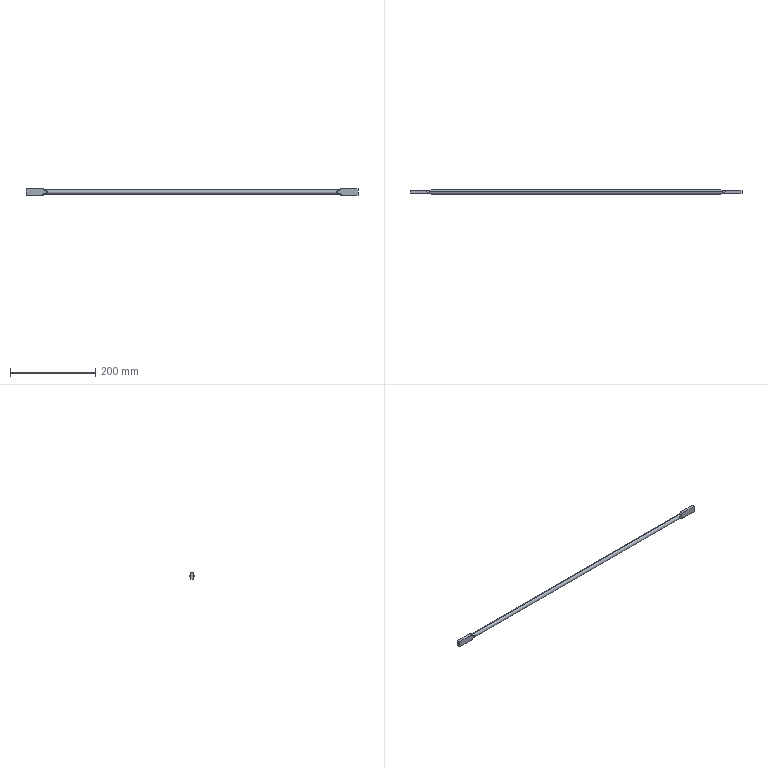Part | SolidWorks | features ICE 2, Extrusion 1, MirrorSolid 1, RevCut 1, Revolution 1 | 1 solid | 22 faces | box 780 x 10 x 15 mm | volume 63253 mm3 | plane 10 | torus 6 | cylinder 6 | commonest cylinder face diameters 18.167 x4 10 x2
STEP:
#1=CARTESIAN_POINT('',(735.,0.,-5.));
#2=VERTEX_POINT('',#1);
#3=CARTESIAN_POINT('',(735.,-3.5,-3.571));
#4=VERTEX_POINT('',#3);
#5=CARTESIAN_POINT('',(735.,0.,0.));
#6=DIRECTION('',(-1.,0.,0.));
#7=DIRECTION('',(0.,0.,1.));
#8=AXIS2_PLACEMENT_3D('',#5,#6,#7);
#9=CIRCLE('',#8,5.);
#10=EDGE_CURVE('',#2,#4,#9,.T.);
#11=ORIENTED_EDGE('',*,*,#10,.F.);
#12=CARTESIAN_POINT('',(740.,0.,-7.5));
#13=VERTEX_POINT('',#12);
#14=CARTESIAN_POINT('',(735.,0.,-11.25));
#15=DIRECTION('',(0.,1.,0.));
#16=DIRECTION('',(0.,0.,1.));
#17=AXIS2_PLACEMENT_3D('',#14,#15,#16);
#18=CIRCLE('',#17,6.25);
#19=EDGE_CURVE('',#2,#13,#18,.T.);
#20=ORIENTED_EDGE('',*,*,#19,.T.);
#21=CARTESIAN_POINT('',(740.497,-3.5,-7.5));
#22=VERTEX_POINT('',#21);
#23=CARTESIAN_POINT('',(740.,0.,-7.5));
#24=CARTESIAN_POINT('',(740.,-0.5937,-7.5));
#25=CARTESIAN_POINT('',(740.055,-1.181,-7.5));
#26=CARTESIAN_POINT('',(740.239,-2.345,-7.5));
#27=CARTESIAN_POINT('',(740.365,-2.923,-7.5));
#28=CARTESIAN_POINT('',(740.497,-3.5,-7.5));
#29=B_SPLINE_CURVE_WITH_KNOTS('',3,(#23,#24,#25,#26,#27,#28),.UNSPECIFIED.,.F.,.F.,(4,2,4),(0.,0.001767,0.003535),.UNSPECIFIED.);
#30=EDGE_CURVE('',#13,#22,#29,.T.);
#31=ORIENTED_EDGE('',*,*,#30,.T.);
#32=CARTESIAN_POINT('',(735.,-3.5,-3.571));
#33=CARTESIAN_POINT('',(735.596,-3.5,-3.571));
#34=CARTESIAN_POINT('',(736.181,-3.5,-3.692));
#35=CARTESIAN_POINT('',(737.291,-3.5,-4.123));
#36=CARTESIAN_POINT('',(737.799,-3.5,-4.42));
#37=CARTESIAN_POINT('',(738.507,-3.5,-4.96));
#38=CARTESIAN_POINT('',(738.732,-3.5,-5.154));
#39=CARTESIAN_POINT('',(739.156,-3.5,-5.567));
#40=CARTESIAN_POINT('',(739.356,-3.5,-5.785));
#41=CARTESIAN_POINT('',(739.732,-3.5,-6.244));
#42=CARTESIAN_POINT('',(739.906,-3.5,-6.485));
#43=CARTESIAN_POINT('',(740.224,-3.5,-6.981));
#44=CARTESIAN_POINT('',(740.368,-3.5,-7.237));
#45=CARTESIAN_POINT('',(740.497,-3.5,-7.5));
#46=B_SPLINE_CURVE_WITH_KNOTS('',3,(#32,#33,#34,#35,#36,#37,#38,#39,#40,#41,#42,#43,#44,#45),.UNSPECIFIED.,.F.,.F.,(4,2,2,2,2,2,4),(0.03499,0.03675,0.03851,0.03939,0.04027,0.04115,0.04203),.UNSPECIFIED.);
#47=EDGE_CURVE('',#4,#22,#46,.T.);
#48=ORIENTED_EDGE('',*,*,#47,.F.);
#49=EDGE_LOOP('',(#11,#20,#31,#48));
#50=FACE_OUTER_BOUND('',#49,.T.);
#51=CARTESIAN_POINT('',(735.,0.,0.));
#52=DIRECTION('',(-1.,0.,0.));
#53=DIRECTION('',(0.,0.,-1.));
#54=AXIS2_PLACEMENT_3D('',#51,#52,#53);
#55=TOROIDAL_SURFACE('',#54,11.25,6.25);
#56=ADVANCED_FACE('',(#50),#55,.F.);
#57=CARTESIAN_POINT('',(45.,3.5,-3.571));
#58=VERTEX_POINT('',#57);
#59=CARTESIAN_POINT('',(45.,0.,-5.));
#60=VERTEX_POINT('',#59);
#61=CARTESIAN_POINT('',(45.,0.,0.));
#62=DIRECTION('',(-1.,0.,0.));
#63=DIRECTION('',(0.,0.,1.));
#64=AXIS2_PLACEMENT_3D('',#61,#62,#63);
#65=CIRCLE('',#64,5.);
#66=EDGE_CURVE('',#58,#60,#65,.T.);
#67=ORIENTED_EDGE('',*,*,#66,.T.);
#68=CARTESIAN_POINT('',(40.,0.,-7.5));
#69=VERTEX_POINT('',#68);
#70=CARTESIAN_POINT('',(45.,0.,-11.25));
#71=DIRECTION('',(0.,-1.,0.));
#72=DIRECTION('',(0.,0.,-1.));
#73=AXIS2_PLACEMENT_3D('',#70,#71,#72);
#74=CIRCLE('',#73,6.25);
#75=EDGE_CURVE('',#60,#69,#74,.T.);
#76=ORIENTED_EDGE('',*,*,#75,.T.);
#77=CARTESIAN_POINT('',(39.503,3.5,-7.5));
#78=VERTEX_POINT('',#77);
#79=CARTESIAN_POINT('',(39.503,3.5,-7.5));
#80=CARTESIAN_POINT('',(39.634,2.924,-7.5));
#81=CARTESIAN_POINT('',(39.761,2.347,-7.5));
#82=CARTESIAN_POINT('',(39.899,1.474,-7.5));
#83=CARTESIAN_POINT('',(39.936,1.182,-7.5));
#84=CARTESIAN_POINT('',(39.974,0.7409,-7.5));
#85=CARTESIAN_POINT('',(39.984,0.5934,-7.5));
#86=CARTESIAN_POINT('',(39.993,0.3715,-7.5));
#87=CARTESIAN_POINT('',(39.997,0.2603,-7.5));
#88=CARTESIAN_POINT('',(39.999,0.1303,-7.5));
#89=CARTESIAN_POINT('',(40.,0.07445,-7.5));
#90=CARTESIAN_POINT('',(40.,0.03724,-7.5));
#91=CARTESIAN_POINT('',(40.,0.01713,-7.5));
#92=CARTESIAN_POINT('',(40.,0.,-7.5));
#93=B_SPLINE_CURVE_WITH_KNOTS('',3,(#79,#80,#81,#82,#83,#84,#85,#86,#87,#88,#89,#90,#91,#92),.UNSPECIFIED.,.F.,.F.,(4,2,2,2,1,1,2,4),(0.07093,0.07256,0.07338,0.07379,0.07399,0.07409,0.07414,0.0742),.UNSPECIFIED.);
#94=EDGE_CURVE('',#78,#69,#93,.T.);
#95=ORIENTED_EDGE('',*,*,#94,.F.);
#96=CARTESIAN_POINT('',(45.,3.5,-3.571));
#97=CARTESIAN_POINT('',(44.404,3.5,-3.571));
#98=CARTESIAN_POINT('',(43.819,3.5,-3.692));
#99=CARTESIAN_POINT('',(42.709,3.5,-4.123));
#100=CARTESIAN_POINT('',(42.201,3.5,-4.42));
#101=CARTESIAN_POINT('',(41.493,3.5,-4.96));
#102=CARTESIAN_POINT('',(41.268,3.5,-5.154));
#103=CARTESIAN_POINT('',(40.844,3.5,-5.567));
#104=CARTESIAN_POINT('',(40.644,3.5,-5.785));
#105=CARTESIAN_POINT('',(40.268,3.5,-6.244));
#106=CARTESIAN_POINT('',(40.094,3.5,-6.485));
#107=CARTESIAN_POINT('',(39.776,3.5,-6.981));
#108=CARTESIAN_POINT('',(39.632,3.5,-7.237));
#109=CARTESIAN_POINT('',(39.503,3.5,-7.5));
#110=B_SPLINE_CURVE_WITH_KNOTS('',3,(#96,#97,#98,#99,#100,#101,#102,#103,#104,#105,#106,#107,#108,#109),.UNSPECIFIED.,.F.,.F.,(4,2,2,2,2,2,4),(0.03499,0.03675,0.03851,0.03939,0.04027,0.04115,0.04203),.UNSPECIFIED.);
#111=EDGE_CURVE('',#58,#78,#110,.T.);
#112=ORIENTED_EDGE('',*,*,#111,.F.);
#113=EDGE_LOOP('',(#67,#76,#95,#112));
#114=FACE_OUTER_BOUND('',#113,.T.);
#115=CARTESIAN_POINT('',(45.,0.,0.));
#116=DIRECTION('',(1.,0.,0.));
#117=DIRECTION('',(0.,0.,-1.));
#118=AXIS2_PLACEMENT_3D('',#115,#116,#117);
#119=TOROIDAL_SURFACE('',#118,11.25,6.25);
#120=ADVANCED_FACE('',(#114),#119,.F.);
#121=CARTESIAN_POINT('',(735.,3.5,-3.571));
#122=VERTEX_POINT('',#121);
#123=CARTESIAN_POINT('',(735.,0.,0.));
#124=DIRECTION('',(-1.,0.,0.));
#125=DIRECTION('',(0.,0.,1.));
#126=AXIS2_PLACEMENT_3D('',#123,#124,#125);
#127=CIRCLE('',#126,5.);
#128=EDGE_CURVE('',#122,#2,#127,.T.);
#129=ORIENTED_EDGE('',*,*,#128,.T.);
#130=CARTESIAN_POINT('',(3.468,0.,-5.));
#131=DIRECTION('',(-1.,0.,0.));
#132=VECTOR('',#131,1000.);
#133=LINE('',#130,#132);
#134=EDGE_CURVE('',#2,#60,#133,.T.);
#135=ORIENTED_EDGE('',*,*,#134,.T.);
#136=ORIENTED_EDGE('',*,*,#66,.F.);
#137=CARTESIAN_POINT('',(45.,3.5,3.571));
#138=VERTEX_POINT('',#137);
#139=CARTESIAN_POINT('',(45.,3.5,-3.571));
#140=CARTESIAN_POINT('',(45.594,3.5,-3.571));
#141=CARTESIAN_POINT('',(46.174,3.558,-3.517));
#142=CARTESIAN_POINT('',(47.025,3.724,-3.338));
#143=CARTESIAN_POINT('',(47.305,3.793,-3.26));
#144=CARTESIAN_POINT('',(47.838,3.95,-3.068));
#145=CARTESIAN_POINT('',(48.093,4.039,-2.953));
#146=CARTESIAN_POINT('',(48.578,4.23,-2.671));
#147=CARTESIAN_POINT('',(48.804,4.332,-2.506));
#148=CARTESIAN_POINT('',(49.208,4.53,-2.126));
#149=CARTESIAN_POINT('',(49.389,4.629,-1.907));
#150=CARTESIAN_POINT('',(49.611,4.757,-1.546));
#151=CARTESIAN_POINT('',(49.677,4.796,-1.42));
#152=CARTESIAN_POINT('',(49.792,4.866,-1.156));
#153=CARTESIAN_POINT('',(49.841,4.897,-1.018));
#154=CARTESIAN_POINT('',(49.959,4.972,-0.5971));
#155=CARTESIAN_POINT('',(49.999,5.,-0.3046));
#156=CARTESIAN_POINT('',(50.001,5.,0.2913));
#157=CARTESIAN_POINT('',(49.962,4.974,0.5826));
#158=CARTESIAN_POINT('',(49.805,4.874,1.151));
#159=CARTESIAN_POINT('',(49.691,4.803,1.414));
#160=CARTESIAN_POINT('',(49.394,4.632,1.901));
#161=CARTESIAN_POINT('',(49.216,4.534,2.118));
#162=CARTESIAN_POINT('',(48.81,4.334,2.502));
#163=CARTESIAN_POINT('',(48.583,4.233,2.667));
#164=CARTESIAN_POINT('',(48.103,4.042,2.947));
#165=CARTESIAN_POINT('',(47.845,3.952,3.065));
#166=CARTESIAN_POINT('',(47.308,3.794,3.259));
#167=CARTESIAN_POINT('',(47.032,3.726,3.336));
#168=CARTESIAN_POINT('',(46.187,3.56,3.515));
#169=CARTESIAN_POINT('',(45.594,3.5,3.571));
#170=CARTESIAN_POINT('',(45.,3.5,3.571));
#171=B_SPLINE_CURVE_WITH_KNOTS('',3,(#139,#140,#141,#142,#143,#144,#145,#146,#147,#148,#149,#150,#151,#152,#153,#154,#155,#156,#157,#158,#159,#160,#161,#162,#163,#164,#165,#166,#167,#168,#169,#170),.UNSPECIFIED.,.F.,.F.,(4,2,2,2,2,2,2,2,2,2,2,2,2,2,2,4),(0.,0.001758,0.002636,0.003515,0.004394,0.005273,0.005712,0.006151,0.00703,0.007909,0.008788,0.009667,0.01055,0.01142,0.0123,0.01406),.UNSPECIFIED.);
#172=EDGE_CURVE('',#58,#138,#171,.T.);
#173=ORIENTED_EDGE('',*,*,#172,.T.);
#174=CARTESIAN_POINT('',(45.,0.,5.));
#175=VERTEX_POINT('',#174);
#176=CARTESIAN_POINT('',(45.,0.,0.));
#177=DIRECTION('',(-1.,0.,0.));
#178=DIRECTION('',(0.,0.,1.));
#179=AXIS2_PLACEMENT_3D('',#176,#177,#178);
#180=CIRCLE('',#179,5.);
#181=EDGE_CURVE('',#175,#138,#180,.T.);
#182=ORIENTED_EDGE('',*,*,#181,.F.);
#183=CARTESIAN_POINT('',(735.,0.,5.));
#184=VERTEX_POINT('',#183);
#185=CARTESIAN_POINT('',(3.468,0.,5.));
#186=DIRECTION('',(-1.,0.,0.));
#187=VECTOR('',#186,1000.);
#188=LINE('',#185,#187);
#189=EDGE_CURVE('',#184,#175,#188,.T.);
#190=ORIENTED_EDGE('',*,*,#189,.F.);
#191=CARTESIAN_POINT('',(735.,3.5,3.571));
#192=VERTEX_POINT('',#191);
#193=CARTESIAN_POINT('',(735.,0.,0.));
#194=DIRECTION('',(-1.,0.,0.));
#195=DIRECTION('',(0.,0.,1.));
#196=AXIS2_PLACEMENT_3D('',#193,#194,#195);
#197=CIRCLE('',#196,5.);
#198=EDGE_CURVE('',#184,#192,#197,.T.);
#199=ORIENTED_EDGE('',*,*,#198,.T.);
#200=CARTESIAN_POINT('',(735.,3.5,-3.571));
#201=CARTESIAN_POINT('',(734.406,3.5,-3.571));
#202=CARTESIAN_POINT('',(733.826,3.558,-3.517));
#203=CARTESIAN_POINT('',(732.975,3.724,-3.338));
#204=CARTESIAN_POINT('',(732.695,3.793,-3.26));
#205=CARTESIAN_POINT('',(732.162,3.95,-3.068));
#206=CARTESIAN_POINT('',(731.907,4.039,-2.953));
#207=CARTESIAN_POINT('',(731.422,4.23,-2.671));
#208=CARTESIAN_POINT('',(731.196,4.332,-2.506));
#209=CARTESIAN_POINT('',(730.792,4.53,-2.126));
#210=CARTESIAN_POINT('',(730.611,4.629,-1.907));
#211=CARTESIAN_POINT('',(730.389,4.757,-1.546));
#212=CARTESIAN_POINT('',(730.323,4.796,-1.42));
#213=CARTESIAN_POINT('',(730.208,4.866,-1.156));
#214=CARTESIAN_POINT('',(730.159,4.897,-1.018));
#215=CARTESIAN_POINT('',(730.041,4.972,-0.5971));
#216=CARTESIAN_POINT('',(730.001,5.,-0.3046));
#217=CARTESIAN_POINT('',(729.999,5.,0.2913));
#218=CARTESIAN_POINT('',(730.038,4.974,0.5826));
#219=CARTESIAN_POINT('',(730.195,4.874,1.151));
#220=CARTESIAN_POINT('',(730.309,4.803,1.414));
#221=CARTESIAN_POINT('',(730.606,4.632,1.901));
#222=CARTESIAN_POINT('',(730.784,4.534,2.118));
#223=CARTESIAN_POINT('',(731.19,4.334,2.502));
#224=CARTESIAN_POINT('',(731.417,4.233,2.667));
#225=CARTESIAN_POINT('',(731.897,4.042,2.947));
#226=CARTESIAN_POINT('',(732.155,3.952,3.065));
#227=CARTESIAN_POINT('',(732.692,3.794,3.259));
#228=CARTESIAN_POINT('',(732.968,3.726,3.336));
#229=CARTESIAN_POINT('',(733.813,3.56,3.515));
#230=CARTESIAN_POINT('',(734.406,3.5,3.571));
#231=CARTESIAN_POINT('',(735.,3.5,3.571));
#232=B_SPLINE_CURVE_WITH_KNOTS('',3,(#200,#201,#202,#203,#204,#205,#206,#207,#208,#209,#210,#211,#212,#213,#214,#215,#216,#217,#218,#219,#220,#221,#222,#223,#224,#225,#226,#227,#228,#229,#230,#231),.UNSPECIFIED.,.F.,.F.,(4,2,2,2,2,2,2,2,2,2,2,2,2,2,2,4),(0.,0.001758,0.002636,0.003515,0.004394,0.005273,0.005712,0.006151,0.00703,0.007909,0.008788,0.009667,0.01055,0.01142,0.0123,0.01406),.UNSPECIFIED.);
#233=EDGE_CURVE('',#122,#192,#232,.T.);
#234=ORIENTED_EDGE('',*,*,#233,.F.);
#235=EDGE_LOOP('',(#129,#135,#136,#173,#182,#190,#199,#234));
#236=FACE_OUTER_BOUND('',#235,.T.);
#237=CARTESIAN_POINT('',(3.468,0.,0.));
#238=DIRECTION('',(-1.,0.,0.));
#239=DIRECTION('',(0.,0.,1.));
#240=AXIS2_PLACEMENT_3D('',#237,#238,#239);
#241=CYLINDRICAL_SURFACE('',#240,5.);
#242=ADVANCED_FACE('',(#236),#241,.T.);
#243=CARTESIAN_POINT('',(0.,-3.5,-7.5));
#244=VERTEX_POINT('',#243);
#245=CARTESIAN_POINT('',(0.,-3.5,7.5));
#246=VERTEX_POINT('',#245);
#247=CARTESIAN_POINT('',(0.,-3.5,7.5));
#248=DIRECTION('',(0.,0.,1.));
#249=VECTOR('',#248,1000.);
#250=LINE('',#247,#249);
#251=EDGE_CURVE('',#244,#246,#250,.T.);
#252=ORIENTED_EDGE('',*,*,#251,.T.);
#253=CARTESIAN_POINT('',(0.,3.5,7.5));
#254=VERTEX_POINT('',#253);
#255=CARTESIAN_POINT('',(0.,3.5,7.5));
#256=DIRECTION('',(0.,-1.,0.));
#257=VECTOR('',#256,1000.);
#258=LINE('',#255,#257);
#259=EDGE_CURVE('',#254,#246,#258,.T.);
#260=ORIENTED_EDGE('',*,*,#259,.F.);
#261=CARTESIAN_POINT('',(0.,3.5,-7.5));
#262=VERTEX_POINT('',#261);
#263=CARTESIAN_POINT('',(0.,3.5,7.5));
#264=DIRECTION('',(0.,0.,1.));
#265=VECTOR('',#264,1000.);
#266=LINE('',#263,#265);
#267=EDGE_CURVE('',#262,#254,#266,.T.);
#268=ORIENTED_EDGE('',*,*,#267,.F.);
#269=CARTESIAN_POINT('',(0.,3.5,-7.5));
#270=DIRECTION('',(0.,-1.,0.));
#271=VECTOR('',#270,1000.);
#272=LINE('',#269,#271);
#273=EDGE_CURVE('',#262,#244,#272,.T.);
#274=ORIENTED_EDGE('',*,*,#273,.T.);
#275=EDGE_LOOP('',(#252,#260,#268,#274));
#276=FACE_OUTER_BOUND('',#275,.T.);
#277=CARTESIAN_POINT('',(0.,3.5,7.5));
#278=DIRECTION('',(1.,0.,0.));
#279=DIRECTION('',(0.,0.,-1.));
#280=AXIS2_PLACEMENT_3D('',#277,#278,#279);
#281=PLANE('',#280);
#282=ADVANCED_FACE('',(#276),#281,.F.);
#283=CARTESIAN_POINT('',(39.503,-3.5,7.5));
#284=VERTEX_POINT('',#283);
#285=CARTESIAN_POINT('',(0.,-3.5,7.5));
#286=DIRECTION('',(1.,0.,0.));
#287=VECTOR('',#286,1000.);
#288=LINE('',#285,#287);
#289=EDGE_CURVE('',#246,#284,#288,.T.);
#290=ORIENTED_EDGE('',*,*,#289,.T.);
#291=CARTESIAN_POINT('',(39.503,3.5,7.5));
#292=VERTEX_POINT('',#291);
#293=CARTESIAN_POINT('',(39.503,-3.5,7.5));
#294=CARTESIAN_POINT('',(39.64,-2.9,7.5));
#295=CARTESIAN_POINT('',(39.771,-2.299,7.5));
#296=CARTESIAN_POINT('',(39.91,-1.389,7.5));
#297=CARTESIAN_POINT('',(39.947,-1.084,7.5));
#298=CARTESIAN_POINT('',(39.982,-0.6242,7.5));
#299=CARTESIAN_POINT('',(39.99,-0.4703,7.5));
#300=CARTESIAN_POINT('',(39.997,-0.2386,7.5));
#301=CARTESIAN_POINT('',(39.999,-0.1612,7.5));
#302=CARTESIAN_POINT('',(40.,-0.04499,7.5));
#303=CARTESIAN_POINT('',(40.,-0.005692,7.5));
#304=CARTESIAN_POINT('',(40.,0.06564,7.5));
#305=CARTESIAN_POINT('',(40.,0.1013,7.5));
#306=CARTESIAN_POINT('',(39.991,0.7068,7.5));
#307=CARTESIAN_POINT('',(39.933,1.27,7.5));
#308=CARTESIAN_POINT('',(39.752,2.39,7.5));
#309=CARTESIAN_POINT('',(39.63,2.945,7.5));
#310=CARTESIAN_POINT('',(39.503,3.5,7.5));
#311=B_SPLINE_CURVE_WITH_KNOTS('',3,(#293,#294,#295,#296,#297,#298,#299,#300,#301,#302,#303,#304,#305,#306,#307,#308,#309,#310),.UNSPECIFIED.,.F.,.F.,(4,2,2,2,2,2,2,2,4),(0.07093,0.07263,0.07348,0.07391,0.07412,0.07423,0.07433,0.07603,0.07773),.UNSPECIFIED.);
#312=EDGE_CURVE('',#284,#292,#311,.T.);
#313=ORIENTED_EDGE('',*,*,#312,.T.);
#314=CARTESIAN_POINT('',(0.,3.5,7.5));
#315=DIRECTION('',(1.,0.,0.));
#316=VECTOR('',#315,1000.);
#317=LINE('',#314,#316);
#318=EDGE_CURVE('',#254,#292,#317,.T.);
#319=ORIENTED_EDGE('',*,*,#318,.F.);
#320=ORIENTED_EDGE('',*,*,#259,.T.);
#321=EDGE_LOOP('',(#290,#313,#319,#320));
#322=FACE_OUTER_BOUND('',#321,.T.);
#323=CARTESIAN_POINT('',(0.,3.5,7.5));
#324=DIRECTION('',(0.,0.,-1.));
#325=DIRECTION('',(-1.,0.,0.));
#326=AXIS2_PLACEMENT_3D('',#323,#324,#325);
#327=PLANE('',#326);
#328=ADVANCED_FACE('',(#322),#327,.F.);
#329=CARTESIAN_POINT('',(0.,3.5,-7.5));
#330=DIRECTION('',(-1.,0.,0.));
#331=VECTOR('',#330,1000.);
#332=LINE('',#329,#331);
#333=EDGE_CURVE('',#78,#262,#332,.T.);
#334=ORIENTED_EDGE('',*,*,#333,.F.);
#335=ORIENTED_EDGE('',*,*,#94,.T.);
#336=CARTESIAN_POINT('',(39.503,-3.5,-7.5));
#337=VERTEX_POINT('',#336);
#338=CARTESIAN_POINT('',(40.,0.,-7.5));
#339=CARTESIAN_POINT('',(40.,-0.5937,-7.5));
#340=CARTESIAN_POINT('',(39.945,-1.181,-7.5));
#341=CARTESIAN_POINT('',(39.761,-2.345,-7.5));
#342=CARTESIAN_POINT('',(39.635,-2.923,-7.5));
#343=CARTESIAN_POINT('',(39.503,-3.5,-7.5));
#344=B_SPLINE_CURVE_WITH_KNOTS('',3,(#338,#339,#340,#341,#342,#343),.UNSPECIFIED.,.F.,.F.,(4,2,4),(0.,0.001767,0.003535),.UNSPECIFIED.);
#345=EDGE_CURVE('',#69,#337,#344,.T.);
#346=ORIENTED_EDGE('',*,*,#345,.T.);
#347=CARTESIAN_POINT('',(0.,-3.5,-7.5));
#348=DIRECTION('',(-1.,0.,0.));
#349=VECTOR('',#348,1000.);
#350=LINE('',#347,#349);
#351=EDGE_CURVE('',#337,#244,#350,.T.);
#352=ORIENTED_EDGE('',*,*,#351,.T.);
#353=ORIENTED_EDGE('',*,*,#273,.F.);
#354=EDGE_LOOP('',(#334,#335,#346,#352,#353));
#355=FACE_OUTER_BOUND('',#354,.T.);
#356=CARTESIAN_POINT('',(0.,3.5,-7.5));
#357=DIRECTION('',(0.,0.,1.));
#358=DIRECTION('',(1.,0.,0.));
#359=AXIS2_PLACEMENT_3D('',#356,#357,#358);
#360=PLANE('',#359);
#361=ADVANCED_FACE('',(#355),#360,.F.);
#362=CARTESIAN_POINT('',(45.,3.5,7.5));
#363=DIRECTION('',(0.,0.,-1.));
#364=VECTOR('',#363,1000.);
#365=LINE('',#362,#364);
#366=EDGE_CURVE('',#138,#58,#365,.T.);
#367=ORIENTED_EDGE('',*,*,#366,.T.);
#368=ORIENTED_EDGE('',*,*,#111,.T.);
#369=ORIENTED_EDGE('',*,*,#333,.T.);
#370=ORIENTED_EDGE('',*,*,#267,.T.);
#371=ORIENTED_EDGE('',*,*,#318,.T.);
#372=CARTESIAN_POINT('',(39.503,3.5,7.5));
#373=CARTESIAN_POINT('',(39.632,3.5,7.236));
#374=CARTESIAN_POINT('',(39.777,3.5,6.979));
#375=CARTESIAN_POINT('',(40.097,3.5,6.481));
#376=CARTESIAN_POINT('',(40.273,3.5,6.239));
#377=CARTESIAN_POINT('',(40.834,3.5,5.552));
#378=CARTESIAN_POINT('',(41.255,3.5,5.141));
#379=CARTESIAN_POINT('',(42.197,3.5,4.424));
#380=CARTESIAN_POINT('',(42.722,3.5,4.117));
#381=CARTESIAN_POINT('',(43.545,3.5,3.799));
#382=CARTESIAN_POINT('',(43.826,3.5,3.716));
#383=CARTESIAN_POINT('',(44.404,3.5,3.601));
#384=CARTESIAN_POINT('',(44.704,3.5,3.571));
#385=CARTESIAN_POINT('',(45.,3.5,3.571));
#386=B_SPLINE_CURVE_WITH_KNOTS('',3,(#372,#373,#374,#375,#376,#377,#378,#379,#380,#381,#382,#383,#384,#385),.UNSPECIFIED.,.F.,.F.,(4,2,2,2,2,2,4),(0.03578,0.03665,0.03753,0.03929,0.04105,0.04193,0.04281),.UNSPECIFIED.);
#387=EDGE_CURVE('',#292,#138,#386,.T.);
#388=ORIENTED_EDGE('',*,*,#387,.T.);
#389=EDGE_LOOP('',(#367,#368,#369,#370,#371,#388));
#390=FACE_OUTER_BOUND('',#389,.T.);
#391=CARTESIAN_POINT('',(0.,3.5,0.));
#392=DIRECTION('',(0.,-1.,0.));
#393=DIRECTION('',(0.,0.,-1.));
#394=AXIS2_PLACEMENT_3D('',#391,#392,#393);
#395=PLANE('',#394);
#396=ADVANCED_FACE('',(#390),#395,.F.);
#397=CARTESIAN_POINT('',(45.,-3.5,-3.571));
#398=VERTEX_POINT('',#397);
#399=CARTESIAN_POINT('',(45.,-3.5,-3.571));
#400=CARTESIAN_POINT('',(44.404,-3.5,-3.571));
#401=CARTESIAN_POINT('',(43.819,-3.5,-3.692));
#402=CARTESIAN_POINT('',(42.709,-3.5,-4.123));
#403=CARTESIAN_POINT('',(42.201,-3.5,-4.42));
#404=CARTESIAN_POINT('',(41.493,-3.5,-4.96));
#405=CARTESIAN_POINT('',(41.268,-3.5,-5.154));
#406=CARTESIAN_POINT('',(40.844,-3.5,-5.567));
#407=CARTESIAN_POINT('',(40.644,-3.5,-5.785));
#408=CARTESIAN_POINT('',(40.268,-3.5,-6.244));
#409=CARTESIAN_POINT('',(40.094,-3.5,-6.485));
#410=CARTESIAN_POINT('',(39.776,-3.5,-6.981));
#411=CARTESIAN_POINT('',(39.632,-3.5,-7.237));
#412=CARTESIAN_POINT('',(39.503,-3.5,-7.5));
#413=B_SPLINE_CURVE_WITH_KNOTS('',3,(#399,#400,#401,#402,#403,#404,#405,#406,#407,#408,#409,#410,#411,#412),.UNSPECIFIED.,.F.,.F.,(4,2,2,2,2,2,4),(0.03499,0.03675,0.03851,0.03939,0.04027,0.04115,0.04203),.UNSPECIFIED.);
#414=EDGE_CURVE('',#398,#337,#413,.T.);
#415=ORIENTED_EDGE('',*,*,#414,.F.);
#416=CARTESIAN_POINT('',(45.,-3.5,3.571));
#417=VERTEX_POINT('',#416);
#418=CARTESIAN_POINT('',(45.,-3.5,7.5));
#419=DIRECTION('',(0.,0.,-1.));
#420=VECTOR('',#419,1000.);
#421=LINE('',#418,#420);
#422=EDGE_CURVE('',#417,#398,#421,.T.);
#423=ORIENTED_EDGE('',*,*,#422,.F.);
#424=CARTESIAN_POINT('',(39.503,-3.5,7.5));
#425=CARTESIAN_POINT('',(39.632,-3.5,7.236));
#426=CARTESIAN_POINT('',(39.777,-3.5,6.979));
#427=CARTESIAN_POINT('',(40.097,-3.5,6.481));
#428=CARTESIAN_POINT('',(40.273,-3.5,6.239));
#429=CARTESIAN_POINT('',(40.834,-3.5,5.552));
#430=CARTESIAN_POINT('',(41.255,-3.5,5.141));
#431=CARTESIAN_POINT('',(42.197,-3.5,4.424));
#432=CARTESIAN_POINT('',(42.722,-3.5,4.117));
#433=CARTESIAN_POINT('',(43.545,-3.5,3.799));
#434=CARTESIAN_POINT('',(43.826,-3.5,3.716));
#435=CARTESIAN_POINT('',(44.404,-3.5,3.601));
#436=CARTESIAN_POINT('',(44.704,-3.5,3.571));
#437=CARTESIAN_POINT('',(45.,-3.5,3.571));
#438=B_SPLINE_CURVE_WITH_KNOTS('',3,(#424,#425,#426,#427,#428,#429,#430,#431,#432,#433,#434,#435,#436,#437),.UNSPECIFIED.,.F.,.F.,(4,2,2,2,2,2,4),(0.03578,0.03665,0.03753,0.03929,0.04105,0.04193,0.04281),.UNSPECIFIED.);
#439=EDGE_CURVE('',#284,#417,#438,.T.);
#440=ORIENTED_EDGE('',*,*,#439,.F.);
#441=ORIENTED_EDGE('',*,*,#289,.F.);
#442=ORIENTED_EDGE('',*,*,#251,.F.);
#443=ORIENTED_EDGE('',*,*,#351,.F.);
#444=EDGE_LOOP('',(#415,#423,#440,#441,#442,#443));
#445=FACE_OUTER_BOUND('',#444,.T.);
#446=CARTESIAN_POINT('',(0.,-3.5,0.));
#447=DIRECTION('',(0.,-1.,0.));
#448=DIRECTION('',(0.,0.,-1.));
#449=AXIS2_PLACEMENT_3D('',#446,#447,#448);
#450=PLANE('',#449);
#451=ADVANCED_FACE('',(#445),#450,.T.);
#452=ORIENTED_EDGE('',*,*,#134,.F.);
#453=ORIENTED_EDGE('',*,*,#10,.T.);
#454=CARTESIAN_POINT('',(735.,-3.5,3.571));
#455=VERTEX_POINT('',#454);
#456=CARTESIAN_POINT('',(735.,-3.5,3.571));
#457=CARTESIAN_POINT('',(734.706,-3.5,3.571));
#458=CARTESIAN_POINT('',(734.409,-3.514,3.557));
#459=CARTESIAN_POINT('',(733.823,-3.572,3.499));
#460=CARTESIAN_POINT('',(733.536,-3.614,3.456));
#461=CARTESIAN_POINT('',(732.974,-3.724,3.337));
#462=CARTESIAN_POINT('',(732.699,-3.792,3.262));
#463=CARTESIAN_POINT('',(732.164,-3.95,3.068));
#464=CARTESIAN_POINT('',(731.904,-4.04,2.951));
#465=CARTESIAN_POINT('',(731.422,-4.23,2.671));
#466=CARTESIAN_POINT('',(731.195,-4.332,2.506));
#467=CARTESIAN_POINT('',(730.788,-4.533,2.122));
#468=CARTESIAN_POINT('',(730.611,-4.629,1.907));
#469=CARTESIAN_POINT('',(730.387,-4.758,1.543));
#470=CARTESIAN_POINT('',(730.321,-4.798,1.414));
#471=CARTESIAN_POINT('',(730.207,-4.867,1.152));
#472=CARTESIAN_POINT('',(730.159,-4.898,1.016));
#473=CARTESIAN_POINT('',(730.041,-4.972,0.5972));
#474=CARTESIAN_POINT('',(730.,-5.,0.2976));
#475=CARTESIAN_POINT('',(730.,-5.,-0.3007));
#476=CARTESIAN_POINT('',(730.04,-4.973,-0.5907));
#477=CARTESIAN_POINT('',(730.157,-4.898,-1.013));
#478=CARTESIAN_POINT('',(730.207,-4.867,-1.152));
#479=CARTESIAN_POINT('',(730.321,-4.798,-1.415));
#480=CARTESIAN_POINT('',(730.386,-4.758,-1.541));
#481=CARTESIAN_POINT('',(730.534,-4.673,-1.782));
#482=CARTESIAN_POINT('',(730.616,-4.627,-1.898));
#483=CARTESIAN_POINT('',(730.794,-4.532,-2.116));
#484=CARTESIAN_POINT('',(730.889,-4.483,-2.218));
#485=CARTESIAN_POINT('',(731.193,-4.333,-2.504));
#486=CARTESIAN_POINT('',(731.422,-4.231,-2.67));
#487=CARTESIAN_POINT('',(731.903,-4.04,-2.951));
#488=CARTESIAN_POINT('',(732.159,-3.951,-3.066));
#489=CARTESIAN_POINT('',(732.694,-3.793,-3.26));
#490=CARTESIAN_POINT('',(732.974,-3.724,-3.337));
#491=CARTESIAN_POINT('',(733.538,-3.614,-3.456));
#492=CARTESIAN_POINT('',(733.825,-3.572,-3.499));
#493=CARTESIAN_POINT('',(734.408,-3.515,-3.557));
#494=CARTESIAN_POINT('',(734.705,-3.5,-3.571));
#495=CARTESIAN_POINT('',(735.,-3.5,-3.571));
#496=B_SPLINE_CURVE_WITH_KNOTS('',3,(#456,#457,#458,#459,#460,#461,#462,#463,#464,#465,#466,#467,#468,#469,#470,#471,#472,#473,#474,#475,#476,#477,#478,#479,#480,#481,#482,#483,#484,#485,#486,#487,#488,#489,#490,#491,#492,#493,#494,#495),.UNSPECIFIED.,.F.,.F.,(4,2,2,2,2,2,2,2,2,2,2,2,2,2,2,2,2,2,2,4),(0.02116,0.02204,0.02293,0.02381,0.02469,0.02557,0.02645,0.02689,0.02733,0.02822,0.0291,0.02954,0.02998,0.03042,0.03086,0.03174,0.03262,0.03351,0.03439,0.03527),.UNSPECIFIED.);
#497=EDGE_CURVE('',#455,#4,#496,.T.);
#498=ORIENTED_EDGE('',*,*,#497,.F.);
#499=CARTESIAN_POINT('',(735.,0.,0.));
#500=DIRECTION('',(-1.,0.,0.));
#501=DIRECTION('',(0.,0.,1.));
#502=AXIS2_PLACEMENT_3D('',#499,#500,#501);
#503=CIRCLE('',#502,5.);
#504=EDGE_CURVE('',#455,#184,#503,.T.);
#505=ORIENTED_EDGE('',*,*,#504,.T.);
#506=ORIENTED_EDGE('',*,*,#189,.T.);
#507=CARTESIAN_POINT('',(45.,0.,0.));
#508=DIRECTION('',(-1.,0.,0.));
#509=DIRECTION('',(0.,0.,1.));
#510=AXIS2_PLACEMENT_3D('',#507,#508,#509);
#511=CIRCLE('',#510,5.);
#512=EDGE_CURVE('',#417,#175,#511,.T.);
#513=ORIENTED_EDGE('',*,*,#512,.F.);
#514=CARTESIAN_POINT('',(45.,-3.5,3.571));
#515=CARTESIAN_POINT('',(45.294,-3.5,3.571));
#516=CARTESIAN_POINT('',(45.591,-3.514,3.557));
#517=CARTESIAN_POINT('',(46.177,-3.572,3.499));
#518=CARTESIAN_POINT('',(46.464,-3.614,3.456));
#519=CARTESIAN_POINT('',(47.026,-3.724,3.337));
#520=CARTESIAN_POINT('',(47.301,-3.792,3.262));
#521=CARTESIAN_POINT('',(47.836,-3.95,3.068));
#522=CARTESIAN_POINT('',(48.096,-4.04,2.951));
#523=CARTESIAN_POINT('',(48.578,-4.23,2.671));
#524=CARTESIAN_POINT('',(48.805,-4.332,2.506));
#525=CARTESIAN_POINT('',(49.212,-4.533,2.122));
#526=CARTESIAN_POINT('',(49.389,-4.629,1.907));
#527=CARTESIAN_POINT('',(49.613,-4.758,1.543));
#528=CARTESIAN_POINT('',(49.679,-4.798,1.414));
#529=CARTESIAN_POINT('',(49.793,-4.867,1.152));
#530=CARTESIAN_POINT('',(49.841,-4.898,1.016));
#531=CARTESIAN_POINT('',(49.959,-4.972,0.5972));
#532=CARTESIAN_POINT('',(50.,-5.,0.2976));
#533=CARTESIAN_POINT('',(50.,-5.,-0.3007));
#534=CARTESIAN_POINT('',(49.96,-4.973,-0.5907));
#535=CARTESIAN_POINT('',(49.843,-4.898,-1.013));
#536=CARTESIAN_POINT('',(49.793,-4.867,-1.152));
#537=CARTESIAN_POINT('',(49.679,-4.798,-1.415));
#538=CARTESIAN_POINT('',(49.614,-4.758,-1.541));
#539=CARTESIAN_POINT('',(49.466,-4.673,-1.782));
#540=CARTESIAN_POINT('',(49.384,-4.627,-1.898));
#541=CARTESIAN_POINT('',(49.206,-4.532,-2.116));
#542=CARTESIAN_POINT('',(49.111,-4.483,-2.218));
#543=CARTESIAN_POINT('',(48.807,-4.333,-2.504));
#544=CARTESIAN_POINT('',(48.578,-4.231,-2.67));
#545=CARTESIAN_POINT('',(48.097,-4.04,-2.951));
#546=CARTESIAN_POINT('',(47.841,-3.951,-3.066));
#547=CARTESIAN_POINT('',(47.306,-3.793,-3.26));
#548=CARTESIAN_POINT('',(47.026,-3.724,-3.337));
#549=CARTESIAN_POINT('',(46.462,-3.614,-3.456));
#550=CARTESIAN_POINT('',(46.175,-3.572,-3.499));
#551=CARTESIAN_POINT('',(45.592,-3.515,-3.557));
#552=CARTESIAN_POINT('',(45.295,-3.5,-3.571));
#553=CARTESIAN_POINT('',(45.,-3.5,-3.571));
#554=B_SPLINE_CURVE_WITH_KNOTS('',3,(#514,#515,#516,#517,#518,#519,#520,#521,#522,#523,#524,#525,#526,#527,#528,#529,#530,#531,#532,#533,#534,#535,#536,#537,#538,#539,#540,#541,#542,#543,#544,#545,#546,#547,#548,#549,#550,#551,#552,#553),.UNSPECIFIED.,.F.,.F.,(4,2,2,2,2,2,2,2,2,2,2,2,2,2,2,2,2,2,2,4),(0.02116,0.02204,0.02293,0.02381,0.02469,0.02557,0.02645,0.02689,0.02733,0.02822,0.0291,0.02954,0.02998,0.03042,0.03086,0.03174,0.03262,0.03351,0.03439,0.03527),.UNSPECIFIED.);
#555=EDGE_CURVE('',#417,#398,#554,.T.);
#556=ORIENTED_EDGE('',*,*,#555,.T.);
#557=CARTESIAN_POINT('',(45.,0.,0.));
#558=DIRECTION('',(-1.,0.,0.));
#559=DIRECTION('',(0.,0.,1.));
#560=AXIS2_PLACEMENT_3D('',#557,#558,#559);
#561=CIRCLE('',#560,5.);
#562=EDGE_CURVE('',#60,#398,#561,.T.);
#563=ORIENTED_EDGE('',*,*,#562,.F.);
#564=EDGE_LOOP('',(#452,#453,#498,#505,#506,#513,#556,#563));
#565=FACE_OUTER_BOUND('',#564,.T.);
#566=CARTESIAN_POINT('',(3.468,0.,0.));
#567=DIRECTION('',(-1.,0.,0.));
#568=DIRECTION('',(0.,0.,1.));
#569=AXIS2_PLACEMENT_3D('',#566,#567,#568);
#570=CYLINDRICAL_SURFACE('',#569,5.);
#571=ADVANCED_FACE('',(#565),#570,.T.);
#572=ORIENTED_EDGE('',*,*,#366,.F.);
#573=ORIENTED_EDGE('',*,*,#172,.F.);
#574=EDGE_LOOP('',(#572,#573));
#575=FACE_OUTER_BOUND('',#574,.T.);
#576=CARTESIAN_POINT('',(45.,12.583,-5.));
#577=DIRECTION('',(0.,0.,1.));
#578=DIRECTION('',(1.,0.,0.));
#579=AXIS2_PLACEMENT_3D('',#576,#577,#578);
#580=CYLINDRICAL_SURFACE('',#579,9.083);
#581=ADVANCED_FACE('',(#575),#580,.F.);
#582=ORIENTED_EDGE('',*,*,#555,.F.);
#583=ORIENTED_EDGE('',*,*,#422,.T.);
#584=EDGE_LOOP('',(#582,#583));
#585=FACE_OUTER_BOUND('',#584,.T.);
#586=CARTESIAN_POINT('',(45.,-12.583,-5.));
#587=DIRECTION('',(0.,0.,1.));
#588=DIRECTION('',(1.,0.,0.));
#589=AXIS2_PLACEMENT_3D('',#586,#587,#588);
#590=CYLINDRICAL_SURFACE('',#589,9.083);
#591=ADVANCED_FACE('',(#585),#590,.F.);
#592=ORIENTED_EDGE('',*,*,#75,.F.);
#593=ORIENTED_EDGE('',*,*,#562,.T.);
#594=ORIENTED_EDGE('',*,*,#414,.T.);
#595=ORIENTED_EDGE('',*,*,#345,.F.);
#596=EDGE_LOOP('',(#592,#593,#594,#595));
#597=FACE_OUTER_BOUND('',#596,.T.);
#598=CARTESIAN_POINT('',(45.,0.,0.));
#599=DIRECTION('',(1.,0.,0.));
#600=DIRECTION('',(0.,0.,-1.));
#601=AXIS2_PLACEMENT_3D('',#598,#599,#600);
#602=TOROIDAL_SURFACE('',#601,11.25,6.25);
#603=ADVANCED_FACE('',(#597),#602,.F.);
#604=ORIENTED_EDGE('',*,*,#312,.F.);
#605=ORIENTED_EDGE('',*,*,#439,.T.);
#606=ORIENTED_EDGE('',*,*,#512,.T.);
#607=ORIENTED_EDGE('',*,*,#181,.T.);
#608=ORIENTED_EDGE('',*,*,#387,.F.);
#609=EDGE_LOOP('',(#604,#605,#606,#607,#608));
#610=FACE_OUTER_BOUND('',#609,.T.);
#611=CARTESIAN_POINT('',(45.,0.,0.));
#612=DIRECTION('',(1.,0.,0.));
#613=DIRECTION('',(0.,0.,-1.));
#614=AXIS2_PLACEMENT_3D('',#611,#612,#613);
#615=TOROIDAL_SURFACE('',#614,11.25,6.25);
#616=ADVANCED_FACE('',(#610),#615,.F.);
#617=CARTESIAN_POINT('',(780.,-3.5,-7.5));
#618=VERTEX_POINT('',#617);
#619=CARTESIAN_POINT('',(780.,-3.5,7.5));
#620=VERTEX_POINT('',#619);
#621=CARTESIAN_POINT('',(780.,-3.5,7.5));
#622=DIRECTION('',(0.,0.,1.));
#623=VECTOR('',#622,1000.);
#624=LINE('',#621,#623);
#625=EDGE_CURVE('',#618,#620,#624,.T.);
#626=ORIENTED_EDGE('',*,*,#625,.F.);
#627=CARTESIAN_POINT('',(780.,3.5,-7.5));
#628=VERTEX_POINT('',#627);
#629=CARTESIAN_POINT('',(780.,3.5,-7.5));
#630=DIRECTION('',(0.,-1.,0.));
#631=VECTOR('',#630,1000.);
#632=LINE('',#629,#631);
#633=EDGE_CURVE('',#628,#618,#632,.T.);
#634=ORIENTED_EDGE('',*,*,#633,.F.);
#635=CARTESIAN_POINT('',(780.,3.5,7.5));
#636=VERTEX_POINT('',#635);
#637=CARTESIAN_POINT('',(780.,3.5,7.5));
#638=DIRECTION('',(0.,0.,1.));
#639=VECTOR('',#638,1000.);
#640=LINE('',#637,#639);
#641=EDGE_CURVE('',#628,#636,#640,.T.);
#642=ORIENTED_EDGE('',*,*,#641,.T.);
#643=CARTESIAN_POINT('',(780.,3.5,7.5));
#644=DIRECTION('',(0.,-1.,0.));
#645=VECTOR('',#644,1000.);
#646=LINE('',#643,#645);
#647=EDGE_CURVE('',#636,#620,#646,.T.);
#648=ORIENTED_EDGE('',*,*,#647,.T.);
#649=EDGE_LOOP('',(#626,#634,#642,#648));
#650=FACE_OUTER_BOUND('',#649,.T.);
#651=CARTESIAN_POINT('',(780.,3.5,7.5));
#652=DIRECTION('',(-1.,0.,0.));
#653=DIRECTION('',(0.,0.,-1.));
#654=AXIS2_PLACEMENT_3D('',#651,#652,#653);
#655=PLANE('',#654);
#656=ADVANCED_FACE('',(#650),#655,.F.);
#657=CARTESIAN_POINT('',(740.497,-3.5,7.5));
#658=VERTEX_POINT('',#657);
#659=CARTESIAN_POINT('',(780.,-3.5,7.5));
#660=DIRECTION('',(-1.,0.,0.));
#661=VECTOR('',#660,1000.);
#662=LINE('',#659,#661);
#663=EDGE_CURVE('',#620,#658,#662,.T.);
#664=ORIENTED_EDGE('',*,*,#663,.F.);
#665=ORIENTED_EDGE('',*,*,#647,.F.);
#666=CARTESIAN_POINT('',(740.497,3.5,7.5));
#667=VERTEX_POINT('',#666);
#668=CARTESIAN_POINT('',(780.,3.5,7.5));
#669=DIRECTION('',(-1.,0.,0.));
#670=VECTOR('',#669,1000.);
#671=LINE('',#668,#670);
#672=EDGE_CURVE('',#636,#667,#671,.T.);
#673=ORIENTED_EDGE('',*,*,#672,.T.);
#674=CARTESIAN_POINT('',(740.497,-3.5,7.5));
#675=CARTESIAN_POINT('',(740.36,-2.9,7.5));
#676=CARTESIAN_POINT('',(740.229,-2.299,7.5));
#677=CARTESIAN_POINT('',(740.09,-1.389,7.5));
#678=CARTESIAN_POINT('',(740.053,-1.084,7.5));
#679=CARTESIAN_POINT('',(740.018,-0.6242,7.5));
#680=CARTESIAN_POINT('',(740.01,-0.4703,7.5));
#681=CARTESIAN_POINT('',(740.003,-0.2386,7.5));
#682=CARTESIAN_POINT('',(740.001,-0.1612,7.5));
#683=CARTESIAN_POINT('',(740.,-0.04499,7.5));
#684=CARTESIAN_POINT('',(740.,-0.005692,7.5));
#685=CARTESIAN_POINT('',(740.,0.06564,7.5));
#686=CARTESIAN_POINT('',(740.,0.1013,7.5));
#687=CARTESIAN_POINT('',(740.009,0.7068,7.5));
#688=CARTESIAN_POINT('',(740.067,1.27,7.5));
#689=CARTESIAN_POINT('',(740.248,2.39,7.5));
#690=CARTESIAN_POINT('',(740.37,2.945,7.5));
#691=CARTESIAN_POINT('',(740.497,3.5,7.5));
#692=B_SPLINE_CURVE_WITH_KNOTS('',3,(#674,#675,#676,#677,#678,#679,#680,#681,#682,#683,#684,#685,#686,#687,#688,#689,#690,#691),.UNSPECIFIED.,.F.,.F.,(4,2,2,2,2,2,2,2,4),(0.07093,0.07263,0.07348,0.07391,0.07412,0.07423,0.07433,0.07603,0.07773),.UNSPECIFIED.);
#693=EDGE_CURVE('',#658,#667,#692,.T.);
#694=ORIENTED_EDGE('',*,*,#693,.F.);
#695=EDGE_LOOP('',(#664,#665,#673,#694));
#696=FACE_OUTER_BOUND('',#695,.T.);
#697=CARTESIAN_POINT('',(780.,3.5,7.5));
#698=DIRECTION('',(0.,0.,-1.));
#699=DIRECTION('',(1.,0.,0.));
#700=AXIS2_PLACEMENT_3D('',#697,#698,#699);
#701=PLANE('',#700);
#702=ADVANCED_FACE('',(#696),#701,.F.);
#703=CARTESIAN_POINT('',(740.497,3.5,-7.5));
#704=VERTEX_POINT('',#703);
#705=CARTESIAN_POINT('',(780.,3.5,-7.5));
#706=DIRECTION('',(1.,0.,0.));
#707=VECTOR('',#706,1000.);
#708=LINE('',#705,#707);
#709=EDGE_CURVE('',#704,#628,#708,.T.);
#710=ORIENTED_EDGE('',*,*,#709,.T.);
#711=ORIENTED_EDGE('',*,*,#633,.T.);
#712=CARTESIAN_POINT('',(780.,-3.5,-7.5));
#713=DIRECTION('',(1.,0.,0.));
#714=VECTOR('',#713,1000.);
#715=LINE('',#712,#714);
#716=EDGE_CURVE('',#22,#618,#715,.T.);
#717=ORIENTED_EDGE('',*,*,#716,.F.);
#718=ORIENTED_EDGE('',*,*,#30,.F.);
#719=CARTESIAN_POINT('',(740.497,3.5,-7.5));
#720=CARTESIAN_POINT('',(740.366,2.924,-7.5));
#721=CARTESIAN_POINT('',(740.239,2.347,-7.5));
#722=CARTESIAN_POINT('',(740.101,1.474,-7.5));
#723=CARTESIAN_POINT('',(740.064,1.182,-7.5));
#724=CARTESIAN_POINT('',(740.026,0.7409,-7.5));
#725=CARTESIAN_POINT('',(740.016,0.5934,-7.5));
#726=CARTESIAN_POINT('',(740.007,0.3715,-7.5));
#727=CARTESIAN_POINT('',(740.003,0.2603,-7.5));
#728=CARTESIAN_POINT('',(740.001,0.1303,-7.5));
#729=CARTESIAN_POINT('',(740.,0.07445,-7.5));
#730=CARTESIAN_POINT('',(740.,0.03724,-7.5));
#731=CARTESIAN_POINT('',(740.,0.01713,-7.5));
#732=CARTESIAN_POINT('',(740.,0.,-7.5));
#733=B_SPLINE_CURVE_WITH_KNOTS('',3,(#719,#720,#721,#722,#723,#724,#725,#726,#727,#728,#729,#730,#731,#732),.UNSPECIFIED.,.F.,.F.,(4,2,2,2,1,1,2,4),(0.07093,0.07256,0.07338,0.07379,0.07399,0.07409,0.07414,0.0742),.UNSPECIFIED.);
#734=EDGE_CURVE('',#704,#13,#733,.T.);
#735=ORIENTED_EDGE('',*,*,#734,.F.);
#736=EDGE_LOOP('',(#710,#711,#717,#718,#735));
#737=FACE_OUTER_BOUND('',#736,.T.);
#738=CARTESIAN_POINT('',(780.,3.5,-7.5));
#739=DIRECTION('',(0.,0.,1.));
#740=DIRECTION('',(-1.,0.,0.));
#741=AXIS2_PLACEMENT_3D('',#738,#739,#740);
#742=PLANE('',#741);
#743=ADVANCED_FACE('',(#737),#742,.F.);
#744=CARTESIAN_POINT('',(735.,3.5,7.5));
#745=DIRECTION('',(0.,0.,-1.));
#746=VECTOR('',#745,1000.);
#747=LINE('',#744,#746);
#748=EDGE_CURVE('',#192,#122,#747,.T.);
#749=ORIENTED_EDGE('',*,*,#748,.F.);
#750=CARTESIAN_POINT('',(740.497,3.5,7.5));
#751=CARTESIAN_POINT('',(740.368,3.5,7.236));
#752=CARTESIAN_POINT('',(740.223,3.5,6.979));
#753=CARTESIAN_POINT('',(739.903,3.5,6.481));
#754=CARTESIAN_POINT('',(739.727,3.5,6.239));
#755=CARTESIAN_POINT('',(739.166,3.5,5.552));
#756=CARTESIAN_POINT('',(738.745,3.5,5.141));
#757=CARTESIAN_POINT('',(737.803,3.5,4.424));
#758=CARTESIAN_POINT('',(737.278,3.5,4.117));
#759=CARTESIAN_POINT('',(736.455,3.5,3.799));
#760=CARTESIAN_POINT('',(736.174,3.5,3.716));
#761=CARTESIAN_POINT('',(735.596,3.5,3.601));
#762=CARTESIAN_POINT('',(735.296,3.5,3.571));
#763=CARTESIAN_POINT('',(735.,3.5,3.571));
#764=B_SPLINE_CURVE_WITH_KNOTS('',3,(#750,#751,#752,#753,#754,#755,#756,#757,#758,#759,#760,#761,#762,#763),.UNSPECIFIED.,.F.,.F.,(4,2,2,2,2,2,4),(0.03578,0.03665,0.03753,0.03929,0.04105,0.04193,0.04281),.UNSPECIFIED.);
#765=EDGE_CURVE('',#667,#192,#764,.T.);
#766=ORIENTED_EDGE('',*,*,#765,.F.);
#767=ORIENTED_EDGE('',*,*,#672,.F.);
#768=ORIENTED_EDGE('',*,*,#641,.F.);
#769=ORIENTED_EDGE('',*,*,#709,.F.);
#770=CARTESIAN_POINT('',(735.,3.5,-3.571));
#771=CARTESIAN_POINT('',(735.596,3.5,-3.571));
#772=CARTESIAN_POINT('',(736.181,3.5,-3.692));
#773=CARTESIAN_POINT('',(737.291,3.5,-4.123));
#774=CARTESIAN_POINT('',(737.799,3.5,-4.42));
#775=CARTESIAN_POINT('',(738.507,3.5,-4.96));
#776=CARTESIAN_POINT('',(738.732,3.5,-5.154));
#777=CARTESIAN_POINT('',(739.156,3.5,-5.567));
#778=CARTESIAN_POINT('',(739.356,3.5,-5.785));
#779=CARTESIAN_POINT('',(739.732,3.5,-6.244));
#780=CARTESIAN_POINT('',(739.906,3.5,-6.485));
#781=CARTESIAN_POINT('',(740.224,3.5,-6.981));
#782=CARTESIAN_POINT('',(740.368,3.5,-7.237));
#783=CARTESIAN_POINT('',(740.497,3.5,-7.5));
#784=B_SPLINE_CURVE_WITH_KNOTS('',3,(#770,#771,#772,#773,#774,#775,#776,#777,#778,#779,#780,#781,#782,#783),.UNSPECIFIED.,.F.,.F.,(4,2,2,2,2,2,4),(0.03499,0.03675,0.03851,0.03939,0.04027,0.04115,0.04203),.UNSPECIFIED.);
#785=EDGE_CURVE('',#122,#704,#784,.T.);
#786=ORIENTED_EDGE('',*,*,#785,.F.);
#787=EDGE_LOOP('',(#749,#766,#767,#768,#769,#786));
#788=FACE_OUTER_BOUND('',#787,.T.);
#789=CARTESIAN_POINT('',(780.,3.5,0.));
#790=DIRECTION('',(0.,-1.,0.));
#791=DIRECTION('',(0.,0.,-1.));
#792=AXIS2_PLACEMENT_3D('',#789,#790,#791);
#793=PLANE('',#792);
#794=ADVANCED_FACE('',(#788),#793,.F.);
#795=ORIENTED_EDGE('',*,*,#47,.T.);
#796=ORIENTED_EDGE('',*,*,#716,.T.);
#797=ORIENTED_EDGE('',*,*,#625,.T.);
#798=ORIENTED_EDGE('',*,*,#663,.T.);
#799=CARTESIAN_POINT('',(740.497,-3.5,7.5));
#800=CARTESIAN_POINT('',(740.368,-3.5,7.236));
#801=CARTESIAN_POINT('',(740.223,-3.5,6.979));
#802=CARTESIAN_POINT('',(739.903,-3.5,6.481));
#803=CARTESIAN_POINT('',(739.727,-3.5,6.239));
#804=CARTESIAN_POINT('',(739.166,-3.5,5.552));
#805=CARTESIAN_POINT('',(738.745,-3.5,5.141));
#806=CARTESIAN_POINT('',(737.803,-3.5,4.424));
#807=CARTESIAN_POINT('',(737.278,-3.5,4.117));
#808=CARTESIAN_POINT('',(736.455,-3.5,3.799));
#809=CARTESIAN_POINT('',(736.174,-3.5,3.716));
#810=CARTESIAN_POINT('',(735.596,-3.5,3.601));
#811=CARTESIAN_POINT('',(735.296,-3.5,3.571));
#812=CARTESIAN_POINT('',(735.,-3.5,3.571));
#813=B_SPLINE_CURVE_WITH_KNOTS('',3,(#799,#800,#801,#802,#803,#804,#805,#806,#807,#808,#809,#810,#811,#812),.UNSPECIFIED.,.F.,.F.,(4,2,2,2,2,2,4),(0.03578,0.03665,0.03753,0.03929,0.04105,0.04193,0.04281),.UNSPECIFIED.);
#814=EDGE_CURVE('',#658,#455,#813,.T.);
#815=ORIENTED_EDGE('',*,*,#814,.T.);
#816=CARTESIAN_POINT('',(735.,-3.5,7.5));
#817=DIRECTION('',(0.,0.,-1.));
#818=VECTOR('',#817,1000.);
#819=LINE('',#816,#818);
#820=EDGE_CURVE('',#455,#4,#819,.T.);
#821=ORIENTED_EDGE('',*,*,#820,.T.);
#822=EDGE_LOOP('',(#795,#796,#797,#798,#815,#821));
#823=FACE_OUTER_BOUND('',#822,.T.);
#824=CARTESIAN_POINT('',(780.,-3.5,0.));
#825=DIRECTION('',(0.,-1.,0.));
#826=DIRECTION('',(0.,0.,-1.));
#827=AXIS2_PLACEMENT_3D('',#824,#825,#826);
#828=PLANE('',#827);
#829=ADVANCED_FACE('',(#823),#828,.T.);
#830=ORIENTED_EDGE('',*,*,#748,.T.);
#831=ORIENTED_EDGE('',*,*,#233,.T.);
#832=EDGE_LOOP('',(#830,#831));
#833=FACE_OUTER_BOUND('',#832,.T.);
#834=CARTESIAN_POINT('',(735.,12.583,-5.));
#835=DIRECTION('',(0.,0.,1.));
#836=DIRECTION('',(-1.,0.,0.));
#837=AXIS2_PLACEMENT_3D('',#834,#835,#836);
#838=CYLINDRICAL_SURFACE('',#837,9.083);
#839=ADVANCED_FACE('',(#833),#838,.F.);
#840=ORIENTED_EDGE('',*,*,#497,.T.);
#841=ORIENTED_EDGE('',*,*,#820,.F.);
#842=EDGE_LOOP('',(#840,#841));
#843=FACE_OUTER_BOUND('',#842,.T.);
#844=CARTESIAN_POINT('',(735.,-12.583,-5.));
#845=DIRECTION('',(0.,0.,1.));
#846=DIRECTION('',(-1.,0.,0.));
#847=AXIS2_PLACEMENT_3D('',#844,#845,#846);
#848=CYLINDRICAL_SURFACE('',#847,9.083);
#849=ADVANCED_FACE('',(#843),#848,.F.);
#850=ORIENTED_EDGE('',*,*,#19,.F.);
#851=ORIENTED_EDGE('',*,*,#128,.F.);
#852=ORIENTED_EDGE('',*,*,#785,.T.);
#853=ORIENTED_EDGE('',*,*,#734,.T.);
#854=EDGE_LOOP('',(#850,#851,#852,#853));
#855=FACE_OUTER_BOUND('',#854,.T.);
#856=CARTESIAN_POINT('',(735.,0.,0.));
#857=DIRECTION('',(-1.,0.,0.));
#858=DIRECTION('',(0.,0.,-1.));
#859=AXIS2_PLACEMENT_3D('',#856,#857,#858);
#860=TOROIDAL_SURFACE('',#859,11.25,6.25);
#861=ADVANCED_FACE('',(#855),#860,.F.);
#862=ORIENTED_EDGE('',*,*,#693,.T.);
#863=ORIENTED_EDGE('',*,*,#765,.T.);
#864=ORIENTED_EDGE('',*,*,#198,.F.);
#865=ORIENTED_EDGE('',*,*,#504,.F.);
#866=ORIENTED_EDGE('',*,*,#814,.F.);
#867=EDGE_LOOP('',(#862,#863,#864,#865,#866));
#868=FACE_OUTER_BOUND('',#867,.T.);
#869=CARTESIAN_POINT('',(735.,0.,0.));
#870=DIRECTION('',(-1.,0.,0.));
#871=DIRECTION('',(0.,0.,-1.));
#872=AXIS2_PLACEMENT_3D('',#869,#870,#871);
#873=TOROIDAL_SURFACE('',#872,11.25,6.25);
#874=ADVANCED_FACE('',(#868),#873,.F.);
#875=CLOSED_SHELL('',(#56,#120,#242,#282,#328,#361,#396,#451,#571,#581,#591,#603,#616,#656,#702,#743,#794,#829,#839,#849,#861,#874));
#876=MANIFOLD_SOLID_BREP('',#875);
#877=CARTESIAN_POINT('',(0.,0.,0.));
#878=DIRECTION('',(0.,0.,1.));
#879=DIRECTION('',(1.,0.,0.));
#880=AXIS2_PLACEMENT_3D('',#877,#878,#879);
#881=(LENGTH_UNIT()NAMED_UNIT(*)SI_UNIT(.MILLI.,.METRE.));
#882=UNCERTAINTY_MEASURE_WITH_UNIT(LENGTH_MEASURE(0.00001),#881,'','');
#883=(NAMED_UNIT(*)PLANE_ANGLE_UNIT()SI_UNIT($,.RADIAN.));
#884=(NAMED_UNIT(*)SI_UNIT($,.STERADIAN.)SOLID_ANGLE_UNIT());
#885=(GEOMETRIC_REPRESENTATION_CONTEXT(3)GLOBAL_UNCERTAINTY_ASSIGNED_CONTEXT((#882))GLOBAL_UNIT_ASSIGNED_CONTEXT((#881,#883,#884))REPRESENTATION_CONTEXT('',''));
#886=ADVANCED_BREP_SHAPE_REPRESENTATION('',(#876,#880),#885);